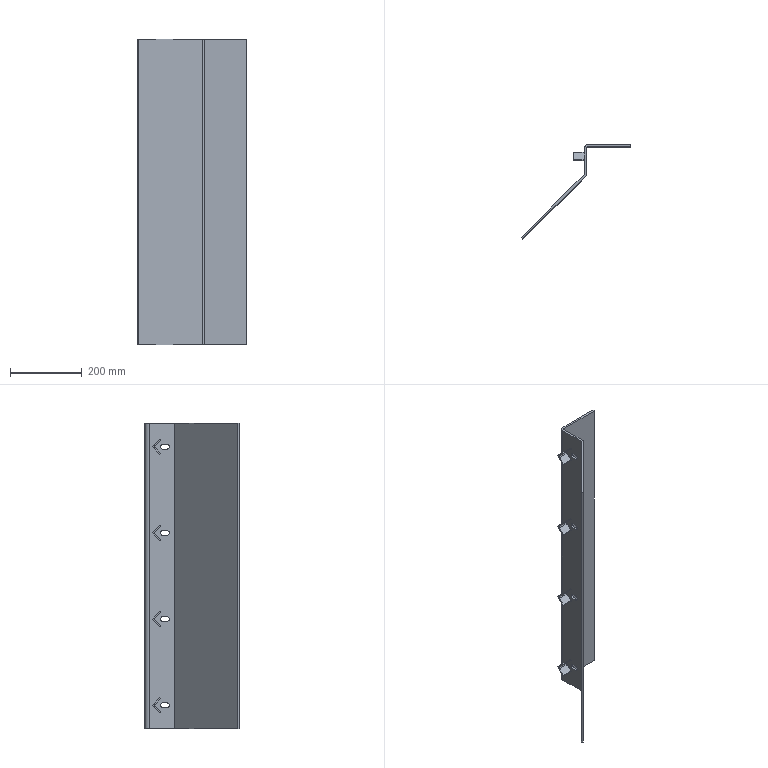Part | STEP file | Beam guard plate_Default<As machined> | 5 solids | 72 faces | box 305.019 x 262.777 x 850 mm | volume 2327560 mm3 | plane 50 | cylinder 22 | commonest cylinder face diameters 2 x8 14 x8 9 x4 12 x1 24 x1